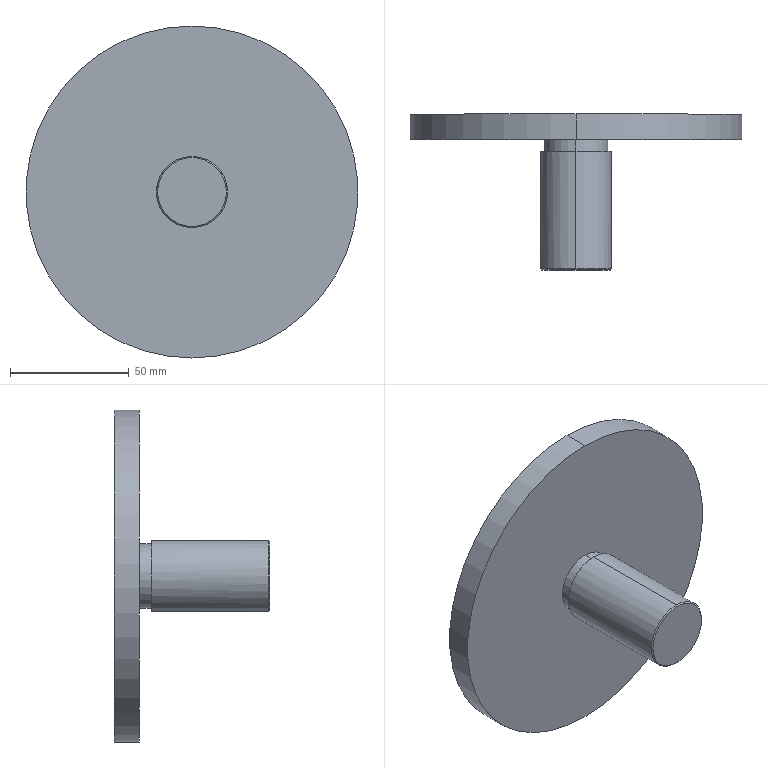Part | SolidWorks | features BaseBody 1 | 1 solid | 12 faces | box 140 x 65.7 x 140 mm | volume 202908 mm3 | cylinder 6 | plane 4 | cone 2 | commonest cylinder face diameters 27 x2 30 x2 140 x2
STEP:
#1=CARTESIAN_POINT('',(0.,10.7,70.));
#2=VERTEX_POINT('',#1);
#3=CARTESIAN_POINT('',(0.,10.7,-70.));
#4=VERTEX_POINT('',#3);
#5=CARTESIAN_POINT('',(0.,10.7,0.));
#6=DIRECTION('',(0.,1.,0.));
#7=DIRECTION('',(0.,0.,-1.));
#8=AXIS2_PLACEMENT_3D('',#5,#6,#7);
#9=CIRCLE('',#8,70.);
#10=EDGE_CURVE('',#2,#4,#9,.T.);
#11=ORIENTED_EDGE('',*,*,#10,.F.);
#12=CARTESIAN_POINT('',(0.,0.,70.));
#13=VERTEX_POINT('',#12);
#14=CARTESIAN_POINT('',(0.,10.7,70.));
#15=DIRECTION('',(0.,-1.,0.));
#16=VECTOR('',#15,1000.);
#17=LINE('',#14,#16);
#18=EDGE_CURVE('',#2,#13,#17,.T.);
#19=ORIENTED_EDGE('',*,*,#18,.T.);
#20=CARTESIAN_POINT('',(0.,0.,-70.));
#21=VERTEX_POINT('',#20);
#22=CARTESIAN_POINT('',(0.,0.,0.));
#23=DIRECTION('',(0.,1.,0.));
#24=DIRECTION('',(0.,0.,-1.));
#25=AXIS2_PLACEMENT_3D('',#22,#23,#24);
#26=CIRCLE('',#25,70.);
#27=EDGE_CURVE('',#13,#21,#26,.T.);
#28=ORIENTED_EDGE('',*,*,#27,.T.);
#29=CARTESIAN_POINT('',(0.,10.7,-70.));
#30=DIRECTION('',(0.,-1.,0.));
#31=VECTOR('',#30,1000.);
#32=LINE('',#29,#31);
#33=EDGE_CURVE('',#4,#21,#32,.T.);
#34=ORIENTED_EDGE('',*,*,#33,.F.);
#35=EDGE_LOOP('',(#11,#19,#28,#34));
#36=FACE_OUTER_BOUND('',#35,.T.);
#37=CARTESIAN_POINT('',(0.,10.7,0.));
#38=DIRECTION('',(0.,-1.,0.));
#39=DIRECTION('',(0.,0.,-1.));
#40=AXIS2_PLACEMENT_3D('',#37,#38,#39);
#41=CYLINDRICAL_SURFACE('',#40,70.);
#42=ADVANCED_FACE('',(#36),#41,.T.);
#43=CARTESIAN_POINT('',(0.,-5.,13.5));
#44=VERTEX_POINT('',#43);
#45=CARTESIAN_POINT('',(0.,-5.,-13.5));
#46=VERTEX_POINT('',#45);
#47=CARTESIAN_POINT('',(0.,-5.,0.));
#48=DIRECTION('',(0.,1.,0.));
#49=DIRECTION('',(0.,0.,1.));
#50=AXIS2_PLACEMENT_3D('',#47,#48,#49);
#51=CIRCLE('',#50,13.5);
#52=EDGE_CURVE('',#44,#46,#51,.T.);
#53=ORIENTED_EDGE('',*,*,#52,.T.);
#54=CARTESIAN_POINT('',(0.,0.,-13.5));
#55=VERTEX_POINT('',#54);
#56=CARTESIAN_POINT('',(0.,-5.,-13.5));
#57=DIRECTION('',(0.,1.,0.));
#58=VECTOR('',#57,1000.);
#59=LINE('',#56,#58);
#60=EDGE_CURVE('',#46,#55,#59,.T.);
#61=ORIENTED_EDGE('',*,*,#60,.T.);
#62=CARTESIAN_POINT('',(0.,0.,13.5));
#63=VERTEX_POINT('',#62);
#64=CARTESIAN_POINT('',(0.,0.,0.));
#65=DIRECTION('',(0.,-1.,0.));
#66=DIRECTION('',(0.,0.,1.));
#67=AXIS2_PLACEMENT_3D('',#64,#65,#66);
#68=CIRCLE('',#67,13.5);
#69=EDGE_CURVE('',#55,#63,#68,.T.);
#70=ORIENTED_EDGE('',*,*,#69,.T.);
#71=CARTESIAN_POINT('',(0.,-5.,13.5));
#72=DIRECTION('',(0.,1.,0.));
#73=VECTOR('',#72,1000.);
#74=LINE('',#71,#73);
#75=EDGE_CURVE('',#44,#63,#74,.T.);
#76=ORIENTED_EDGE('',*,*,#75,.F.);
#77=EDGE_LOOP('',(#53,#61,#70,#76));
#78=FACE_OUTER_BOUND('',#77,.T.);
#79=CARTESIAN_POINT('',(0.,-5.,0.));
#80=DIRECTION('',(0.,1.,0.));
#81=DIRECTION('',(0.,0.,1.));
#82=AXIS2_PLACEMENT_3D('',#79,#80,#81);
#83=CYLINDRICAL_SURFACE('',#82,13.5);
#84=ADVANCED_FACE('',(#78),#83,.T.);
#85=CARTESIAN_POINT('',(15.,-54.5,0.));
#86=VERTEX_POINT('',#85);
#87=CARTESIAN_POINT('',(0.,-54.5,-15.));
#88=VERTEX_POINT('',#87);
#89=CARTESIAN_POINT('',(0.,-54.5,0.));
#90=DIRECTION('',(0.,1.,0.));
#91=DIRECTION('',(0.,0.,1.));
#92=AXIS2_PLACEMENT_3D('',#89,#90,#91);
#93=CIRCLE('',#92,15.);
#94=EDGE_CURVE('',#86,#88,#93,.T.);
#95=ORIENTED_EDGE('',*,*,#94,.T.);
#96=CARTESIAN_POINT('',(0.,-5.,-15.));
#97=VERTEX_POINT('',#96);
#98=CARTESIAN_POINT('',(0.,-55.,-15.));
#99=DIRECTION('',(0.,1.,0.));
#100=VECTOR('',#99,1000.);
#101=LINE('',#98,#100);
#102=EDGE_CURVE('',#88,#97,#101,.T.);
#103=ORIENTED_EDGE('',*,*,#102,.T.);
#104=CARTESIAN_POINT('',(0.,-5.,15.));
#105=VERTEX_POINT('',#104);
#106=CARTESIAN_POINT('',(0.,-5.,0.));
#107=DIRECTION('',(0.,-1.,0.));
#108=DIRECTION('',(0.,0.,1.));
#109=AXIS2_PLACEMENT_3D('',#106,#107,#108);
#110=CIRCLE('',#109,15.);
#111=EDGE_CURVE('',#97,#105,#110,.T.);
#112=ORIENTED_EDGE('',*,*,#111,.T.);
#113=CARTESIAN_POINT('',(0.,-54.5,15.));
#114=VERTEX_POINT('',#113);
#115=CARTESIAN_POINT('',(0.,-55.,15.));
#116=DIRECTION('',(0.,1.,0.));
#117=VECTOR('',#116,1000.);
#118=LINE('',#115,#117);
#119=EDGE_CURVE('',#114,#105,#118,.T.);
#120=ORIENTED_EDGE('',*,*,#119,.F.);
#121=CARTESIAN_POINT('',(0.,-54.5,0.));
#122=DIRECTION('',(0.,1.,0.));
#123=DIRECTION('',(0.,0.,1.));
#124=AXIS2_PLACEMENT_3D('',#121,#122,#123);
#125=CIRCLE('',#124,15.);
#126=EDGE_CURVE('',#114,#86,#125,.T.);
#127=ORIENTED_EDGE('',*,*,#126,.T.);
#128=EDGE_LOOP('',(#95,#103,#112,#120,#127));
#129=FACE_OUTER_BOUND('',#128,.T.);
#130=CARTESIAN_POINT('',(0.,-55.,0.));
#131=DIRECTION('',(0.,1.,0.));
#132=DIRECTION('',(0.,0.,1.));
#133=AXIS2_PLACEMENT_3D('',#130,#131,#132);
#134=CYLINDRICAL_SURFACE('',#133,15.);
#135=ADVANCED_FACE('',(#129),#134,.T.);
#136=CARTESIAN_POINT('',(-14.5,-55.,0.));
#137=VERTEX_POINT('',#136);
#138=CARTESIAN_POINT('',(14.5,-55.,0.));
#139=VERTEX_POINT('',#138);
#140=CARTESIAN_POINT('',(0.,-55.,0.));
#141=DIRECTION('',(0.,1.,0.));
#142=DIRECTION('',(-1.,0.,0.));
#143=AXIS2_PLACEMENT_3D('',#140,#141,#142);
#144=CIRCLE('',#143,14.5);
#145=EDGE_CURVE('',#137,#139,#144,.T.);
#146=ORIENTED_EDGE('',*,*,#145,.T.);
#147=CARTESIAN_POINT('',(15.,-54.5,0.));
#148=DIRECTION('',(0.7071,0.7071,0.));
#149=VECTOR('',#148,1000.);
#150=LINE('',#147,#149);
#151=EDGE_CURVE('',#139,#86,#150,.T.);
#152=ORIENTED_EDGE('',*,*,#151,.T.);
#153=ORIENTED_EDGE('',*,*,#126,.F.);
#154=CARTESIAN_POINT('',(-15.,-54.5,0.));
#155=VERTEX_POINT('',#154);
#156=CARTESIAN_POINT('',(0.,-54.5,0.));
#157=DIRECTION('',(0.,1.,0.));
#158=DIRECTION('',(0.,0.,1.));
#159=AXIS2_PLACEMENT_3D('',#156,#157,#158);
#160=CIRCLE('',#159,15.);
#161=EDGE_CURVE('',#155,#114,#160,.T.);
#162=ORIENTED_EDGE('',*,*,#161,.F.);
#163=CARTESIAN_POINT('',(-15.,-54.5,0.));
#164=DIRECTION('',(-0.7071,0.7071,0.));
#165=VECTOR('',#164,1000.);
#166=LINE('',#163,#165);
#167=EDGE_CURVE('',#137,#155,#166,.T.);
#168=ORIENTED_EDGE('',*,*,#167,.F.);
#169=EDGE_LOOP('',(#146,#152,#153,#162,#168));
#170=FACE_OUTER_BOUND('',#169,.T.);
#171=CARTESIAN_POINT('',(0.,-54.5,0.));
#172=DIRECTION('',(0.,1.,0.));
#173=DIRECTION('',(-1.,0.,0.));
#174=AXIS2_PLACEMENT_3D('',#171,#172,#173);
#175=CONICAL_SURFACE('',#174,15.,0.7854);
#176=ADVANCED_FACE('',(#170),#175,.T.);
#177=CARTESIAN_POINT('',(0.,10.7,0.));
#178=DIRECTION('',(0.,1.,0.));
#179=DIRECTION('',(0.,0.,-1.));
#180=AXIS2_PLACEMENT_3D('',#177,#178,#179);
#181=CIRCLE('',#180,70.);
#182=EDGE_CURVE('',#4,#2,#181,.T.);
#183=ORIENTED_EDGE('',*,*,#182,.T.);
#184=ORIENTED_EDGE('',*,*,#10,.T.);
#185=EDGE_LOOP('',(#183,#184));
#186=FACE_OUTER_BOUND('',#185,.T.);
#187=CARTESIAN_POINT('',(0.,10.7,0.));
#188=DIRECTION('',(0.,1.,0.));
#189=DIRECTION('',(0.,0.,1.));
#190=AXIS2_PLACEMENT_3D('',#187,#188,#189);
#191=PLANE('',#190);
#192=ADVANCED_FACE('',(#186),#191,.T.);
#193=ORIENTED_EDGE('',*,*,#18,.F.);
#194=ORIENTED_EDGE('',*,*,#182,.F.);
#195=ORIENTED_EDGE('',*,*,#33,.T.);
#196=CARTESIAN_POINT('',(0.,0.,0.));
#197=DIRECTION('',(0.,1.,0.));
#198=DIRECTION('',(0.,0.,-1.));
#199=AXIS2_PLACEMENT_3D('',#196,#197,#198);
#200=CIRCLE('',#199,70.);
#201=EDGE_CURVE('',#21,#13,#200,.T.);
#202=ORIENTED_EDGE('',*,*,#201,.T.);
#203=EDGE_LOOP('',(#193,#194,#195,#202));
#204=FACE_OUTER_BOUND('',#203,.T.);
#205=CARTESIAN_POINT('',(0.,10.7,0.));
#206=DIRECTION('',(0.,-1.,0.));
#207=DIRECTION('',(0.,0.,-1.));
#208=AXIS2_PLACEMENT_3D('',#205,#206,#207);
#209=CYLINDRICAL_SURFACE('',#208,70.);
#210=ADVANCED_FACE('',(#204),#209,.T.);
#211=ORIENTED_EDGE('',*,*,#201,.F.);
#212=ORIENTED_EDGE('',*,*,#27,.F.);
#213=EDGE_LOOP('',(#211,#212));
#214=FACE_OUTER_BOUND('',#213,.T.);
#215=CARTESIAN_POINT('',(0.,0.,0.));
#216=DIRECTION('',(0.,-1.,0.));
#217=DIRECTION('',(0.,0.,1.));
#218=AXIS2_PLACEMENT_3D('',#215,#216,#217);
#219=CIRCLE('',#218,13.5);
#220=EDGE_CURVE('',#63,#55,#219,.T.);
#221=ORIENTED_EDGE('',*,*,#220,.F.);
#222=ORIENTED_EDGE('',*,*,#69,.F.);
#223=EDGE_LOOP('',(#221,#222));
#224=FACE_BOUND('',#223,.T.);
#225=CARTESIAN_POINT('',(0.,0.,0.));
#226=DIRECTION('',(0.,1.,0.));
#227=DIRECTION('',(0.,0.,1.));
#228=AXIS2_PLACEMENT_3D('',#225,#226,#227);
#229=PLANE('',#228);
#230=ADVANCED_FACE('',(#214,#224),#229,.F.);
#231=ORIENTED_EDGE('',*,*,#60,.F.);
#232=CARTESIAN_POINT('',(0.,-5.,0.));
#233=DIRECTION('',(0.,1.,0.));
#234=DIRECTION('',(0.,0.,1.));
#235=AXIS2_PLACEMENT_3D('',#232,#233,#234);
#236=CIRCLE('',#235,13.5);
#237=EDGE_CURVE('',#46,#44,#236,.T.);
#238=ORIENTED_EDGE('',*,*,#237,.T.);
#239=ORIENTED_EDGE('',*,*,#75,.T.);
#240=ORIENTED_EDGE('',*,*,#220,.T.);
#241=EDGE_LOOP('',(#231,#238,#239,#240));
#242=FACE_OUTER_BOUND('',#241,.T.);
#243=CARTESIAN_POINT('',(0.,-5.,0.));
#244=DIRECTION('',(0.,1.,0.));
#245=DIRECTION('',(0.,0.,1.));
#246=AXIS2_PLACEMENT_3D('',#243,#244,#245);
#247=CYLINDRICAL_SURFACE('',#246,13.5);
#248=ADVANCED_FACE('',(#242),#247,.T.);
#249=CARTESIAN_POINT('',(0.,-5.,0.));
#250=DIRECTION('',(0.,-1.,0.));
#251=DIRECTION('',(0.,0.,1.));
#252=AXIS2_PLACEMENT_3D('',#249,#250,#251);
#253=CIRCLE('',#252,15.);
#254=EDGE_CURVE('',#105,#97,#253,.T.);
#255=ORIENTED_EDGE('',*,*,#254,.F.);
#256=ORIENTED_EDGE('',*,*,#111,.F.);
#257=EDGE_LOOP('',(#255,#256));
#258=FACE_OUTER_BOUND('',#257,.T.);
#259=ORIENTED_EDGE('',*,*,#52,.F.);
#260=ORIENTED_EDGE('',*,*,#237,.F.);
#261=EDGE_LOOP('',(#259,#260));
#262=FACE_BOUND('',#261,.T.);
#263=CARTESIAN_POINT('',(0.,-5.,0.));
#264=DIRECTION('',(0.,-1.,0.));
#265=DIRECTION('',(0.,0.,-1.));
#266=AXIS2_PLACEMENT_3D('',#263,#264,#265);
#267=PLANE('',#266);
#268=ADVANCED_FACE('',(#258,#262),#267,.F.);
#269=ORIENTED_EDGE('',*,*,#102,.F.);
#270=CARTESIAN_POINT('',(0.,-54.5,0.));
#271=DIRECTION('',(0.,1.,0.));
#272=DIRECTION('',(0.,0.,1.));
#273=AXIS2_PLACEMENT_3D('',#270,#271,#272);
#274=CIRCLE('',#273,15.);
#275=EDGE_CURVE('',#88,#155,#274,.T.);
#276=ORIENTED_EDGE('',*,*,#275,.T.);
#277=ORIENTED_EDGE('',*,*,#161,.T.);
#278=ORIENTED_EDGE('',*,*,#119,.T.);
#279=ORIENTED_EDGE('',*,*,#254,.T.);
#280=EDGE_LOOP('',(#269,#276,#277,#278,#279));
#281=FACE_OUTER_BOUND('',#280,.T.);
#282=CARTESIAN_POINT('',(0.,-55.,0.));
#283=DIRECTION('',(0.,1.,0.));
#284=DIRECTION('',(0.,0.,1.));
#285=AXIS2_PLACEMENT_3D('',#282,#283,#284);
#286=CYLINDRICAL_SURFACE('',#285,15.);
#287=ADVANCED_FACE('',(#281),#286,.T.);
#288=ORIENTED_EDGE('',*,*,#151,.F.);
#289=CARTESIAN_POINT('',(0.,-55.,0.));
#290=DIRECTION('',(0.,1.,0.));
#291=DIRECTION('',(-1.,0.,0.));
#292=AXIS2_PLACEMENT_3D('',#289,#290,#291);
#293=CIRCLE('',#292,14.5);
#294=EDGE_CURVE('',#139,#137,#293,.T.);
#295=ORIENTED_EDGE('',*,*,#294,.T.);
#296=ORIENTED_EDGE('',*,*,#167,.T.);
#297=ORIENTED_EDGE('',*,*,#275,.F.);
#298=ORIENTED_EDGE('',*,*,#94,.F.);
#299=EDGE_LOOP('',(#288,#295,#296,#297,#298));
#300=FACE_OUTER_BOUND('',#299,.T.);
#301=CARTESIAN_POINT('',(0.,-54.5,0.));
#302=DIRECTION('',(0.,1.,0.));
#303=DIRECTION('',(-1.,0.,0.));
#304=AXIS2_PLACEMENT_3D('',#301,#302,#303);
#305=CONICAL_SURFACE('',#304,15.,0.7854);
#306=ADVANCED_FACE('',(#300),#305,.T.);
#307=ORIENTED_EDGE('',*,*,#145,.F.);
#308=ORIENTED_EDGE('',*,*,#294,.F.);
#309=EDGE_LOOP('',(#307,#308));
#310=FACE_OUTER_BOUND('',#309,.T.);
#311=CARTESIAN_POINT('',(0.,-55.,0.));
#312=DIRECTION('',(0.,-1.,0.));
#313=DIRECTION('',(0.,0.,-1.));
#314=AXIS2_PLACEMENT_3D('',#311,#312,#313);
#315=PLANE('',#314);
#316=ADVANCED_FACE('',(#310),#315,.T.);
#317=CLOSED_SHELL('',(#42,#84,#135,#176,#192,#210,#230,#248,#268,#287,#306,#316));
#318=MANIFOLD_SOLID_BREP('',#317);
#319=CARTESIAN_POINT('',(0.,0.,0.));
#320=DIRECTION('',(0.,0.,1.));
#321=DIRECTION('',(1.,0.,0.));
#322=AXIS2_PLACEMENT_3D('',#319,#320,#321);
#323=(LENGTH_UNIT()NAMED_UNIT(*)SI_UNIT(.MILLI.,.METRE.));
#324=UNCERTAINTY_MEASURE_WITH_UNIT(LENGTH_MEASURE(0.00001),#323,'','');
#325=(NAMED_UNIT(*)PLANE_ANGLE_UNIT()SI_UNIT($,.RADIAN.));
#326=(NAMED_UNIT(*)SI_UNIT($,.STERADIAN.)SOLID_ANGLE_UNIT());
#327=(GEOMETRIC_REPRESENTATION_CONTEXT(3)GLOBAL_UNCERTAINTY_ASSIGNED_CONTEXT((#324))GLOBAL_UNIT_ASSIGNED_CONTEXT((#323,#325,#326))REPRESENTATION_CONTEXT('',''));
#328=ADVANCED_BREP_SHAPE_REPRESENTATION('',(#318,#322),#327);